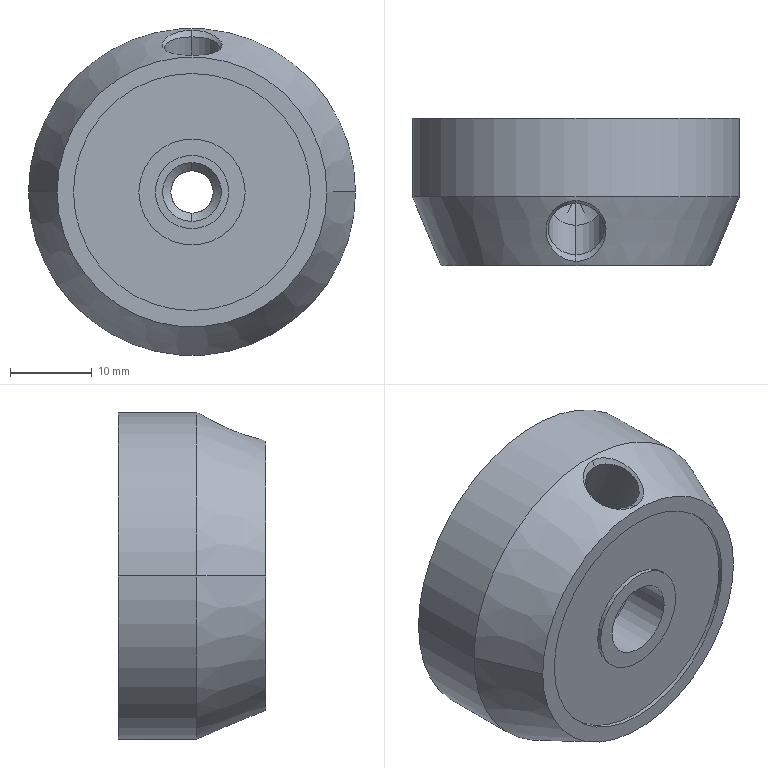Part | SolidWorks | features ICE 8, Chamfer 1, ExtruRefSurface 1, HoleWzd 1, Revolution 1 | 1 solid | 48 faces | box 40 x 18 x 40 mm | volume 16236 mm3 | cylinder 27 | plane 13 | cone 8 | commonest cylinder face diameters 6 x4 5 x3 5.2 x2 6.8 x2 7 x2 8 x2
STEP:
#1=CARTESIAN_POINT('',(20.,2.785,10.327));
#2=VERTEX_POINT('',#1);
#3=CARTESIAN_POINT('',(20.,-3.492,7.712));
#4=VERTEX_POINT('',#3);
#5=CARTESIAN_POINT('',(20.,-0.3538,9.019));
#6=DIRECTION('',(0.,-0.3846,0.9231));
#7=DIRECTION('',(0.,-0.9231,-0.3846));
#8=AXIS2_PLACEMENT_3D('',#5,#6,#7);
#9=CIRCLE('',#8,3.4);
#10=EDGE_CURVE('',#2,#4,#9,.T.);
#11=ORIENTED_EDGE('',*,*,#10,.F.);
#12=CARTESIAN_POINT('',(20.,-0.8212,18.981));
#13=VERTEX_POINT('',#12);
#14=CARTESIAN_POINT('',(20.,-1.062,19.558));
#15=DIRECTION('',(0.,-0.3846,0.9231));
#16=VECTOR('',#15,1000.);
#17=LINE('',#14,#16);
#18=EDGE_CURVE('',#2,#13,#17,.T.);
#19=ORIENTED_EDGE('',*,*,#18,.T.);
#20=CARTESIAN_POINT('',(20.,-7.098,16.365));
#21=VERTEX_POINT('',#20);
#22=CARTESIAN_POINT('',(20.,-3.96,17.673));
#23=DIRECTION('',(0.,-0.3846,0.9231));
#24=DIRECTION('',(0.,-0.9231,-0.3846));
#25=AXIS2_PLACEMENT_3D('',#22,#23,#24);
#26=CIRCLE('',#25,3.4);
#27=EDGE_CURVE('',#13,#21,#26,.T.);
#28=ORIENTED_EDGE('',*,*,#27,.T.);
#29=CARTESIAN_POINT('',(20.,-7.338,16.942));
#30=DIRECTION('',(0.,-0.3846,0.9231));
#31=VECTOR('',#30,1000.);
#32=LINE('',#29,#31);
#33=EDGE_CURVE('',#4,#21,#32,.T.);
#34=ORIENTED_EDGE('',*,*,#33,.F.);
#35=EDGE_LOOP('',(#11,#19,#28,#34));
#36=FACE_OUTER_BOUND('',#35,.T.);
#37=CARTESIAN_POINT('',(20.,-4.2,18.25));
#38=DIRECTION('',(0.,-0.3846,0.9231));
#39=DIRECTION('',(0.,-0.9231,-0.3846));
#40=AXIS2_PLACEMENT_3D('',#37,#38,#39);
#41=CYLINDRICAL_SURFACE('',#40,3.4);
#42=ADVANCED_FACE('',(#36),#41,.F.);
#43=CARTESIAN_POINT('',(20.,0.4319,7.133));
#44=VERTEX_POINT('',#43);
#45=CARTESIAN_POINT('',(20.,-3.492,7.712));
#46=DIRECTION('',(0.,-0.9893,0.1457));
#47=VECTOR('',#46,1000.);
#48=LINE('',#45,#47);
#49=EDGE_CURVE('',#44,#4,#48,.T.);
#50=ORIENTED_EDGE('',*,*,#49,.F.);
#51=CARTESIAN_POINT('',(20.,2.785,10.327));
#52=DIRECTION('',(0.,0.5931,0.8051));
#53=VECTOR('',#52,1000.);
#54=LINE('',#51,#53);
#55=EDGE_CURVE('',#44,#2,#54,.T.);
#56=ORIENTED_EDGE('',*,*,#55,.T.);
#57=ORIENTED_EDGE('',*,*,#10,.T.);
#58=EDGE_LOOP('',(#50,#56,#57));
#59=FACE_OUTER_BOUND('',#58,.T.);
#60=CARTESIAN_POINT('',(20.,-0.3538,9.019));
#61=DIRECTION('',(0.,-0.3846,0.9231));
#62=DIRECTION('',(0.,-0.9231,-0.3846));
#63=AXIS2_PLACEMENT_3D('',#60,#61,#62);
#64=CONICAL_SURFACE('',#63,3.4,1.03);
#65=ADVANCED_FACE('',(#59),#64,.F.);
#66=ORIENTED_EDGE('',*,*,#27,.F.);
#67=CARTESIAN_POINT('',(20.,-0.4846,19.798));
#68=VERTEX_POINT('',#67);
#69=CARTESIAN_POINT('',(20.,-0.4846,19.798));
#70=DIRECTION('',(0.,0.3807,0.9247));
#71=VECTOR('',#70,1000.);
#72=LINE('',#69,#71);
#73=EDGE_CURVE('',#13,#68,#72,.T.);
#74=ORIENTED_EDGE('',*,*,#73,.T.);
#75=CARTESIAN_POINT('',(20.,-7.915,16.702));
#76=VERTEX_POINT('',#75);
#77=CARTESIAN_POINT('',(20.,-7.915,16.702));
#78=CARTESIAN_POINT('',(19.748,-7.915,16.702));
#79=CARTESIAN_POINT('',(19.492,-7.886,16.708));
#80=CARTESIAN_POINT('',(19.001,-7.772,16.734));
#81=CARTESIAN_POINT('',(18.762,-7.688,16.753));
#82=CARTESIAN_POINT('',(18.304,-7.469,16.804));
#83=CARTESIAN_POINT('',(18.091,-7.338,16.836));
#84=CARTESIAN_POINT('',(17.693,-7.035,16.913));
#85=CARTESIAN_POINT('',(17.508,-6.863,16.959));
#86=CARTESIAN_POINT('',(17.176,-6.492,17.064));
#87=CARTESIAN_POINT('',(17.029,-6.292,17.123));
#88=CARTESIAN_POINT('',(16.776,-5.877,17.253));
#89=CARTESIAN_POINT('',(16.67,-5.66,17.324));
#90=CARTESIAN_POINT('',(16.497,-5.211,17.481));
#91=CARTESIAN_POINT('',(16.431,-4.98,17.566));
#92=CARTESIAN_POINT('',(16.343,-4.518,17.745));
#93=CARTESIAN_POINT('',(16.321,-4.286,17.839));
#94=CARTESIAN_POINT('',(16.319,-3.818,18.037));
#95=CARTESIAN_POINT('',(16.341,-3.587,18.14));
#96=CARTESIAN_POINT('',(16.427,-3.139,18.348));
#97=CARTESIAN_POINT('',(16.491,-2.919,18.453));
#98=CARTESIAN_POINT('',(16.665,-2.491,18.667));
#99=CARTESIAN_POINT('',(16.772,-2.288,18.772));
#100=CARTESIAN_POINT('',(17.025,-1.906,18.975));
#101=CARTESIAN_POINT('',(17.173,-1.725,19.074));
#102=CARTESIAN_POINT('',(17.508,-1.391,19.26));
#103=CARTESIAN_POINT('',(17.691,-1.242,19.346));
#104=CARTESIAN_POINT('',(18.089,-0.9786,19.5));
#105=CARTESIAN_POINT('',(18.307,-0.863,19.569));
#106=CARTESIAN_POINT('',(18.764,-0.6766,19.681));
#107=CARTESIAN_POINT('',(19.001,-0.6058,19.724));
#108=CARTESIAN_POINT('',(19.492,-0.5095,19.783));
#109=CARTESIAN_POINT('',(19.748,-0.4846,19.798));
#110=CARTESIAN_POINT('',(20.,-0.4846,19.798));
#111=B_SPLINE_CURVE_WITH_KNOTS('',3,(#77,#78,#79,#80,#81,#82,#83,#84,#85,#86,#87,#88,#89,#90,#91,#92,#93,#94,#95,#96,#97,#98,#99,#100,#101,#102,#103,#104,#105,#106,#107,#108,#109,#110),.UNSPECIFIED.,.F.,.F.,(4,2,2,2,2,2,2,2,2,2,2,2,2,2,2,2,4),(0.02082,0.02157,0.02232,0.02308,0.02383,0.02458,0.02534,0.02609,0.02684,0.0276,0.02835,0.0291,0.02986,0.03061,0.03136,0.03212,0.03287),.UNSPECIFIED.);
#112=EDGE_CURVE('',#76,#68,#111,.T.);
#113=ORIENTED_EDGE('',*,*,#112,.F.);
#114=CARTESIAN_POINT('',(20.,-7.915,16.702));
#115=DIRECTION('',(0.,-0.9247,0.3807));
#116=VECTOR('',#115,1000.);
#117=LINE('',#114,#116);
#118=EDGE_CURVE('',#21,#76,#117,.T.);
#119=ORIENTED_EDGE('',*,*,#118,.F.);
#120=EDGE_LOOP('',(#66,#74,#113,#119));
#121=FACE_OUTER_BOUND('',#120,.T.);
#122=CARTESIAN_POINT('',(20.,-4.2,18.25));
#123=DIRECTION('',(0.,-0.3846,0.9231));
#124=DIRECTION('',(0.,-0.9231,-0.3846));
#125=AXIS2_PLACEMENT_3D('',#122,#123,#124);
#126=CONICAL_SURFACE('',#125,4.025,0.7854);
#127=ADVANCED_FACE('',(#121),#126,.F.);
#128=CARTESIAN_POINT('',(26.5,-7.9,0.));
#129=VERTEX_POINT('',#128);
#130=CARTESIAN_POINT('',(13.5,-7.9,0.));
#131=VERTEX_POINT('',#130);
#132=CARTESIAN_POINT('',(20.,-7.9,0.));
#133=DIRECTION('',(0.,-1.,0.));
#134=DIRECTION('',(1.,0.,0.));
#135=AXIS2_PLACEMENT_3D('',#132,#133,#134);
#136=CIRCLE('',#135,6.5);
#137=EDGE_CURVE('',#129,#131,#136,.T.);
#138=ORIENTED_EDGE('',*,*,#137,.T.);
#139=CARTESIAN_POINT('',(13.5,-8.4,0.));
#140=VERTEX_POINT('',#139);
#141=CARTESIAN_POINT('',(13.5,-7.9,0.));
#142=DIRECTION('',(0.,-1.,0.));
#143=VECTOR('',#142,1000.);
#144=LINE('',#141,#143);
#145=EDGE_CURVE('',#131,#140,#144,.T.);
#146=ORIENTED_EDGE('',*,*,#145,.T.);
#147=CARTESIAN_POINT('',(26.5,-8.4,0.));
#148=VERTEX_POINT('',#147);
#149=CARTESIAN_POINT('',(20.,-8.4,0.));
#150=DIRECTION('',(0.,-1.,0.));
#151=DIRECTION('',(1.,0.,0.));
#152=AXIS2_PLACEMENT_3D('',#149,#150,#151);
#153=CIRCLE('',#152,6.5);
#154=EDGE_CURVE('',#148,#140,#153,.T.);
#155=ORIENTED_EDGE('',*,*,#154,.F.);
#156=CARTESIAN_POINT('',(26.5,-7.9,0.));
#157=DIRECTION('',(0.,-1.,0.));
#158=VECTOR('',#157,1000.);
#159=LINE('',#156,#158);
#160=EDGE_CURVE('',#129,#148,#159,.T.);
#161=ORIENTED_EDGE('',*,*,#160,.F.);
#162=EDGE_LOOP('',(#138,#146,#155,#161));
#163=FACE_OUTER_BOUND('',#162,.T.);
#164=CARTESIAN_POINT('',(20.,-7.9,0.));
#165=DIRECTION('',(0.,-1.,0.));
#166=DIRECTION('',(1.,0.,0.));
#167=AXIS2_PLACEMENT_3D('',#164,#165,#166);
#168=CYLINDRICAL_SURFACE('',#167,6.5);
#169=ADVANCED_FACE('',(#163),#168,.T.);
#170=CARTESIAN_POINT('',(5.5,-7.9,0.));
#171=VERTEX_POINT('',#170);
#172=CARTESIAN_POINT('',(34.5,-7.9,0.));
#173=VERTEX_POINT('',#172);
#174=CARTESIAN_POINT('',(20.,-7.9,0.));
#175=DIRECTION('',(0.,-1.,0.));
#176=DIRECTION('',(1.,0.,0.));
#177=AXIS2_PLACEMENT_3D('',#174,#175,#176);
#178=CIRCLE('',#177,14.5);
#179=EDGE_CURVE('',#171,#173,#178,.T.);
#180=ORIENTED_EDGE('',*,*,#179,.F.);
#181=CARTESIAN_POINT('',(5.5,-8.4,0.));
#182=VERTEX_POINT('',#181);
#183=CARTESIAN_POINT('',(5.5,-7.9,0.));
#184=DIRECTION('',(0.,-1.,0.));
#185=VECTOR('',#184,1000.);
#186=LINE('',#183,#185);
#187=EDGE_CURVE('',#171,#182,#186,.T.);
#188=ORIENTED_EDGE('',*,*,#187,.T.);
#189=CARTESIAN_POINT('',(34.5,-8.4,0.));
#190=VERTEX_POINT('',#189);
#191=CARTESIAN_POINT('',(20.,-8.4,0.));
#192=DIRECTION('',(0.,-1.,0.));
#193=DIRECTION('',(1.,0.,0.));
#194=AXIS2_PLACEMENT_3D('',#191,#192,#193);
#195=CIRCLE('',#194,14.5);
#196=EDGE_CURVE('',#182,#190,#195,.T.);
#197=ORIENTED_EDGE('',*,*,#196,.T.);
#198=CARTESIAN_POINT('',(34.5,-7.9,0.));
#199=DIRECTION('',(0.,-1.,0.));
#200=VECTOR('',#199,1000.);
#201=LINE('',#198,#200);
#202=EDGE_CURVE('',#173,#190,#201,.T.);
#203=ORIENTED_EDGE('',*,*,#202,.F.);
#204=EDGE_LOOP('',(#180,#188,#197,#203));
#205=FACE_OUTER_BOUND('',#204,.T.);
#206=CARTESIAN_POINT('',(20.,-7.9,0.));
#207=DIRECTION('',(0.,-1.,0.));
#208=DIRECTION('',(1.,0.,0.));
#209=AXIS2_PLACEMENT_3D('',#206,#207,#208);
#210=CYLINDRICAL_SURFACE('',#209,14.5);
#211=ADVANCED_FACE('',(#205),#210,.F.);
#212=CARTESIAN_POINT('',(20.,-1.4,2.6));
#213=VERTEX_POINT('',#212);
#214=CARTESIAN_POINT('',(17.4,-1.4,0.));
#215=VERTEX_POINT('',#214);
#216=CARTESIAN_POINT('',(20.,-1.4,0.));
#217=DIRECTION('',(0.,-1.,0.));
#218=DIRECTION('',(0.,0.,-1.));
#219=AXIS2_PLACEMENT_3D('',#216,#217,#218);
#220=CIRCLE('',#219,2.6);
#221=EDGE_CURVE('',#213,#215,#220,.T.);
#222=ORIENTED_EDGE('',*,*,#221,.F.);
#223=CARTESIAN_POINT('',(20.,-2.4,3.6));
#224=VERTEX_POINT('',#223);
#225=CARTESIAN_POINT('',(20.,-1.4,2.6));
#226=DIRECTION('',(0.,-0.7071,0.7071));
#227=VECTOR('',#226,1000.);
#228=LINE('',#225,#227);
#229=EDGE_CURVE('',#213,#224,#228,.T.);
#230=ORIENTED_EDGE('',*,*,#229,.T.);
#231=CARTESIAN_POINT('',(20.,-2.4,-3.6));
#232=VERTEX_POINT('',#231);
#233=CARTESIAN_POINT('',(20.,-2.4,0.));
#234=DIRECTION('',(0.,1.,0.));
#235=DIRECTION('',(1.,0.,0.));
#236=AXIS2_PLACEMENT_3D('',#233,#234,#235);
#237=CIRCLE('',#236,3.6);
#238=EDGE_CURVE('',#232,#224,#237,.T.);
#239=ORIENTED_EDGE('',*,*,#238,.F.);
#240=CARTESIAN_POINT('',(20.,-1.4,-2.6));
#241=VERTEX_POINT('',#240);
#242=CARTESIAN_POINT('',(20.,-1.4,-2.6));
#243=DIRECTION('',(0.,-0.7071,-0.7071));
#244=VECTOR('',#243,1000.);
#245=LINE('',#242,#244);
#246=EDGE_CURVE('',#241,#232,#245,.T.);
#247=ORIENTED_EDGE('',*,*,#246,.F.);
#248=CARTESIAN_POINT('',(20.,-1.4,0.));
#249=DIRECTION('',(0.,-1.,0.));
#250=DIRECTION('',(0.,0.,-1.));
#251=AXIS2_PLACEMENT_3D('',#248,#249,#250);
#252=CIRCLE('',#251,2.6);
#253=EDGE_CURVE('',#215,#241,#252,.T.);
#254=ORIENTED_EDGE('',*,*,#253,.F.);
#255=EDGE_LOOP('',(#222,#230,#239,#247,#254));
#256=FACE_OUTER_BOUND('',#255,.T.);
#257=CARTESIAN_POINT('',(20.,-1.4,0.));
#258=DIRECTION('',(0.,-1.,0.));
#259=DIRECTION('',(0.,0.,-1.));
#260=AXIS2_PLACEMENT_3D('',#257,#258,#259);
#261=CONICAL_SURFACE('',#260,2.6,0.7854);
#262=ADVANCED_FACE('',(#256),#261,.F.);
#263=ORIENTED_EDGE('',*,*,#253,.T.);
#264=CARTESIAN_POINT('',(22.6,-1.4,0.));
#265=VERTEX_POINT('',#264);
#266=CARTESIAN_POINT('',(20.,-1.4,0.));
#267=DIRECTION('',(0.,-1.,0.));
#268=DIRECTION('',(0.,0.,-1.));
#269=AXIS2_PLACEMENT_3D('',#266,#267,#268);
#270=CIRCLE('',#269,2.6);
#271=EDGE_CURVE('',#241,#265,#270,.T.);
#272=ORIENTED_EDGE('',*,*,#271,.T.);
#273=CARTESIAN_POINT('',(22.6,0.6,0.));
#274=VERTEX_POINT('',#273);
#275=CARTESIAN_POINT('',(22.6,-8.4,0.));
#276=DIRECTION('',(0.,1.,0.));
#277=VECTOR('',#276,1000.);
#278=LINE('',#275,#277);
#279=EDGE_CURVE('',#265,#274,#278,.T.);
#280=ORIENTED_EDGE('',*,*,#279,.T.);
#281=CARTESIAN_POINT('',(17.4,0.6,0.));
#282=VERTEX_POINT('',#281);
#283=CARTESIAN_POINT('',(20.,0.6,0.));
#284=DIRECTION('',(0.,1.,0.));
#285=DIRECTION('',(-1.,0.,0.));
#286=AXIS2_PLACEMENT_3D('',#283,#284,#285);
#287=CIRCLE('',#286,2.6);
#288=EDGE_CURVE('',#274,#282,#287,.T.);
#289=ORIENTED_EDGE('',*,*,#288,.T.);
#290=CARTESIAN_POINT('',(17.4,-8.4,0.));
#291=DIRECTION('',(0.,1.,0.));
#292=VECTOR('',#291,1000.);
#293=LINE('',#290,#292);
#294=EDGE_CURVE('',#215,#282,#293,.T.);
#295=ORIENTED_EDGE('',*,*,#294,.F.);
#296=EDGE_LOOP('',(#263,#272,#280,#289,#295));
#297=FACE_OUTER_BOUND('',#296,.T.);
#298=CARTESIAN_POINT('',(20.,-8.4,0.));
#299=DIRECTION('',(0.,1.,0.));
#300=DIRECTION('',(-1.,0.,0.));
#301=AXIS2_PLACEMENT_3D('',#298,#299,#300);
#302=CYLINDRICAL_SURFACE('',#301,2.6);
#303=ADVANCED_FACE('',(#297),#302,.F.);
#304=CARTESIAN_POINT('',(23.5,0.6,0.));
#305=VERTEX_POINT('',#304);
#306=CARTESIAN_POINT('',(16.5,0.6,0.));
#307=VERTEX_POINT('',#306);
#308=CARTESIAN_POINT('',(20.,0.6,0.));
#309=DIRECTION('',(0.,1.,0.));
#310=DIRECTION('',(-1.,0.,0.));
#311=AXIS2_PLACEMENT_3D('',#308,#309,#310);
#312=CIRCLE('',#311,3.5);
#313=EDGE_CURVE('',#305,#307,#312,.T.);
#314=ORIENTED_EDGE('',*,*,#313,.F.);
#315=CARTESIAN_POINT('',(23.5,3.1,0.));
#316=VERTEX_POINT('',#315);
#317=CARTESIAN_POINT('',(23.5,0.6,0.));
#318=DIRECTION('',(0.,1.,0.));
#319=VECTOR('',#318,1000.);
#320=LINE('',#317,#319);
#321=EDGE_CURVE('',#305,#316,#320,.T.);
#322=ORIENTED_EDGE('',*,*,#321,.T.);
#323=CARTESIAN_POINT('',(16.5,3.1,0.));
#324=VERTEX_POINT('',#323);
#325=CARTESIAN_POINT('',(20.,3.1,0.));
#326=DIRECTION('',(0.,1.,0.));
#327=DIRECTION('',(-1.,0.,0.));
#328=AXIS2_PLACEMENT_3D('',#325,#326,#327);
#329=CIRCLE('',#328,3.5);
#330=EDGE_CURVE('',#316,#324,#329,.T.);
#331=ORIENTED_EDGE('',*,*,#330,.T.);
#332=CARTESIAN_POINT('',(16.5,0.6,0.));
#333=DIRECTION('',(0.,1.,0.));
#334=VECTOR('',#333,1000.);
#335=LINE('',#332,#334);
#336=EDGE_CURVE('',#307,#324,#335,.T.);
#337=ORIENTED_EDGE('',*,*,#336,.F.);
#338=EDGE_LOOP('',(#314,#322,#331,#337));
#339=FACE_OUTER_BOUND('',#338,.T.);
#340=CARTESIAN_POINT('',(20.,0.6,0.));
#341=DIRECTION('',(0.,1.,0.));
#342=DIRECTION('',(-1.,0.,0.));
#343=AXIS2_PLACEMENT_3D('',#340,#341,#342);
#344=CYLINDRICAL_SURFACE('',#343,3.5);
#345=ADVANCED_FACE('',(#339),#344,.F.);
#346=CARTESIAN_POINT('',(15.5,-2.4,0.));
#347=VERTEX_POINT('',#346);
#348=CARTESIAN_POINT('',(24.5,-2.4,0.));
#349=VERTEX_POINT('',#348);
#350=CARTESIAN_POINT('',(20.,-2.4,0.));
#351=DIRECTION('',(0.,-1.,0.));
#352=DIRECTION('',(1.,0.,0.));
#353=AXIS2_PLACEMENT_3D('',#350,#351,#352);
#354=CIRCLE('',#353,4.5);
#355=EDGE_CURVE('',#347,#349,#354,.T.);
#356=ORIENTED_EDGE('',*,*,#355,.F.);
#357=CARTESIAN_POINT('',(15.5,-8.4,0.));
#358=VERTEX_POINT('',#357);
#359=CARTESIAN_POINT('',(15.5,-2.4,0.));
#360=DIRECTION('',(0.,-1.,0.));
#361=VECTOR('',#360,1000.);
#362=LINE('',#359,#361);
#363=EDGE_CURVE('',#347,#358,#362,.T.);
#364=ORIENTED_EDGE('',*,*,#363,.T.);
#365=CARTESIAN_POINT('',(24.5,-8.4,0.));
#366=VERTEX_POINT('',#365);
#367=CARTESIAN_POINT('',(20.,-8.4,0.));
#368=DIRECTION('',(0.,-1.,0.));
#369=DIRECTION('',(1.,0.,0.));
#370=AXIS2_PLACEMENT_3D('',#367,#368,#369);
#371=CIRCLE('',#370,4.5);
#372=EDGE_CURVE('',#358,#366,#371,.T.);
#373=ORIENTED_EDGE('',*,*,#372,.T.);
#374=CARTESIAN_POINT('',(24.5,-2.4,0.));
#375=DIRECTION('',(0.,-1.,0.));
#376=VECTOR('',#375,1000.);
#377=LINE('',#374,#376);
#378=EDGE_CURVE('',#349,#366,#377,.T.);
#379=ORIENTED_EDGE('',*,*,#378,.F.);
#380=EDGE_LOOP('',(#356,#364,#373,#379));
#381=FACE_OUTER_BOUND('',#380,.T.);
#382=CARTESIAN_POINT('',(20.,-2.4,0.));
#383=DIRECTION('',(0.,-1.,0.));
#384=DIRECTION('',(1.,0.,0.));
#385=AXIS2_PLACEMENT_3D('',#382,#383,#384);
#386=CYLINDRICAL_SURFACE('',#385,4.5);
#387=ADVANCED_FACE('',(#381),#386,.F.);
#388=CARTESIAN_POINT('',(9.,-3.4,0.));
#389=VERTEX_POINT('',#388);
#390=CARTESIAN_POINT('',(3.,-3.4,0.));
#391=VERTEX_POINT('',#390);
#392=CARTESIAN_POINT('',(6.,-3.4,0.));
#393=DIRECTION('',(0.,1.,0.));
#394=DIRECTION('',(-1.,0.,0.));
#395=AXIS2_PLACEMENT_3D('',#392,#393,#394);
#396=CIRCLE('',#395,3.);
#397=EDGE_CURVE('',#389,#391,#396,.T.);
#398=ORIENTED_EDGE('',*,*,#397,.F.);
#399=CARTESIAN_POINT('',(9.,7.6,0.));
#400=VERTEX_POINT('',#399);
#401=CARTESIAN_POINT('',(9.,-3.4,0.));
#402=DIRECTION('',(0.,1.,0.));
#403=VECTOR('',#402,1000.);
#404=LINE('',#401,#403);
#405=EDGE_CURVE('',#389,#400,#404,.T.);
#406=ORIENTED_EDGE('',*,*,#405,.T.);
#407=CARTESIAN_POINT('',(3.,7.6,0.));
#408=VERTEX_POINT('',#407);
#409=CARTESIAN_POINT('',(6.,7.6,0.));
#410=DIRECTION('',(0.,1.,0.));
#411=DIRECTION('',(-1.,0.,0.));
#412=AXIS2_PLACEMENT_3D('',#409,#410,#411);
#413=CIRCLE('',#412,3.);
#414=EDGE_CURVE('',#400,#408,#413,.T.);
#415=ORIENTED_EDGE('',*,*,#414,.T.);
#416=CARTESIAN_POINT('',(3.,-3.4,0.));
#417=DIRECTION('',(0.,1.,0.));
#418=VECTOR('',#417,1000.);
#419=LINE('',#416,#418);
#420=EDGE_CURVE('',#391,#408,#419,.T.);
#421=ORIENTED_EDGE('',*,*,#420,.F.);
#422=EDGE_LOOP('',(#398,#406,#415,#421));
#423=FACE_OUTER_BOUND('',#422,.T.);
#424=CARTESIAN_POINT('',(6.,-3.4,0.));
#425=DIRECTION('',(0.,1.,0.));
#426=DIRECTION('',(-1.,0.,0.));
#427=AXIS2_PLACEMENT_3D('',#424,#425,#426);
#428=CYLINDRICAL_SURFACE('',#427,3.);
#429=ADVANCED_FACE('',(#423),#428,.F.);
#430=CARTESIAN_POINT('',(37.,-3.4,0.));
#431=VERTEX_POINT('',#430);
#432=CARTESIAN_POINT('',(31.,-3.4,0.));
#433=VERTEX_POINT('',#432);
#434=CARTESIAN_POINT('',(34.,-3.4,0.));
#435=DIRECTION('',(0.,1.,0.));
#436=DIRECTION('',(1.,0.,0.));
#437=AXIS2_PLACEMENT_3D('',#434,#435,#436);
#438=CIRCLE('',#437,3.);
#439=EDGE_CURVE('',#431,#433,#438,.T.);
#440=ORIENTED_EDGE('',*,*,#439,.F.);
#441=CARTESIAN_POINT('',(37.,7.6,0.));
#442=VERTEX_POINT('',#441);
#443=CARTESIAN_POINT('',(37.,-3.4,0.));
#444=DIRECTION('',(0.,1.,0.));
#445=VECTOR('',#444,1000.);
#446=LINE('',#443,#445);
#447=EDGE_CURVE('',#431,#442,#446,.T.);
#448=ORIENTED_EDGE('',*,*,#447,.T.);
#449=CARTESIAN_POINT('',(31.,7.6,0.));
#450=VERTEX_POINT('',#449);
#451=CARTESIAN_POINT('',(34.,7.6,0.));
#452=DIRECTION('',(0.,1.,0.));
#453=DIRECTION('',(1.,0.,0.));
#454=AXIS2_PLACEMENT_3D('',#451,#452,#453);
#455=CIRCLE('',#454,3.);
#456=EDGE_CURVE('',#442,#450,#455,.T.);
#457=ORIENTED_EDGE('',*,*,#456,.T.);
#458=CARTESIAN_POINT('',(31.,-3.4,0.));
#459=DIRECTION('',(0.,1.,0.));
#460=VECTOR('',#459,1000.);
#461=LINE('',#458,#460);
#462=EDGE_CURVE('',#433,#450,#461,.T.);
#463=ORIENTED_EDGE('',*,*,#462,.F.);
#464=EDGE_LOOP('',(#440,#448,#457,#463));
#465=FACE_OUTER_BOUND('',#464,.T.);
#466=CARTESIAN_POINT('',(34.,-3.4,0.));
#467=DIRECTION('',(0.,1.,0.));
#468=DIRECTION('',(-1.,0.,0.));
#469=AXIS2_PLACEMENT_3D('',#466,#467,#468);
#470=CYLINDRICAL_SURFACE('',#469,3.);
#471=ADVANCED_FACE('',(#465),#470,.F.);
#472=CARTESIAN_POINT('',(7.601,4.1,-9.899));
#473=VERTEX_POINT('',#472);
#474=CARTESIAN_POINT('',(11.868,4.1,-8.132));
#475=VERTEX_POINT('',#474);
#476=CARTESIAN_POINT('',(10.101,4.1,-9.899));
#477=DIRECTION('',(0.,1.,0.));
#478=DIRECTION('',(-1.,0.,0.));
#479=AXIS2_PLACEMENT_3D('',#476,#477,#478);
#480=CIRCLE('',#479,2.5);
#481=EDGE_CURVE('',#473,#475,#480,.T.);
#482=ORIENTED_EDGE('',*,*,#481,.F.);
#483=CARTESIAN_POINT('',(7.601,7.6,-9.899));
#484=VERTEX_POINT('',#483);
#485=CARTESIAN_POINT('',(7.601,4.1,-9.899));
#486=DIRECTION('',(0.,1.,0.));
#487=VECTOR('',#486,1000.);
#488=LINE('',#485,#487);
#489=EDGE_CURVE('',#473,#484,#488,.T.);
#490=ORIENTED_EDGE('',*,*,#489,.T.);
#491=CARTESIAN_POINT('',(11.868,7.6,-8.132));
#492=VERTEX_POINT('',#491);
#493=CARTESIAN_POINT('',(10.101,7.6,-9.899));
#494=DIRECTION('',(0.,1.,0.));
#495=DIRECTION('',(-1.,0.,0.));
#496=AXIS2_PLACEMENT_3D('',#493,#494,#495);
#497=CIRCLE('',#496,2.5);
#498=EDGE_CURVE('',#484,#492,#497,.T.);
#499=ORIENTED_EDGE('',*,*,#498,.T.);
#500=CARTESIAN_POINT('',(11.868,4.1,-8.132));
#501=DIRECTION('',(0.,1.,0.));
#502=VECTOR('',#501,1000.);
#503=LINE('',#500,#502);
#504=EDGE_CURVE('',#475,#492,#503,.T.);
#505=ORIENTED_EDGE('',*,*,#504,.F.);
#506=EDGE_LOOP('',(#482,#490,#499,#505));
#507=FACE_OUTER_BOUND('',#506,.T.);
#508=CARTESIAN_POINT('',(10.101,4.1,-9.899));
#509=DIRECTION('',(0.,1.,0.));
#510=DIRECTION('',(-1.,0.,0.));
#511=AXIS2_PLACEMENT_3D('',#508,#509,#510);
#512=CYLINDRICAL_SURFACE('',#511,2.5);
#513=ADVANCED_FACE('',(#507),#512,.F.);
#514=CARTESIAN_POINT('',(20.,7.6,0.));
#515=DIRECTION('',(0.,1.,0.));
#516=DIRECTION('',(-1.,0.,0.));
#517=AXIS2_PLACEMENT_3D('',#514,#515,#516);
#518=CIRCLE('',#517,17.);
#519=EDGE_CURVE('',#442,#408,#518,.T.);
#520=ORIENTED_EDGE('',*,*,#519,.F.);
#521=CARTESIAN_POINT('',(37.,9.6,0.));
#522=VERTEX_POINT('',#521);
#523=CARTESIAN_POINT('',(37.,7.6,0.));
#524=DIRECTION('',(0.,1.,0.));
#525=VECTOR('',#524,1000.);
#526=LINE('',#523,#525);
#527=EDGE_CURVE('',#442,#522,#526,.T.);
#528=ORIENTED_EDGE('',*,*,#527,.T.);
#529=CARTESIAN_POINT('',(3.,9.6,0.));
#530=VERTEX_POINT('',#529);
#531=CARTESIAN_POINT('',(20.,9.6,0.));
#532=DIRECTION('',(0.,1.,0.));
#533=DIRECTION('',(-1.,0.,0.));
#534=AXIS2_PLACEMENT_3D('',#531,#532,#533);
#535=CIRCLE('',#534,17.);
#536=EDGE_CURVE('',#522,#530,#535,.T.);
#537=ORIENTED_EDGE('',*,*,#536,.T.);
#538=CARTESIAN_POINT('',(3.,7.6,0.));
#539=DIRECTION('',(0.,1.,0.));
#540=VECTOR('',#539,1000.);
#541=LINE('',#538,#540);
#542=EDGE_CURVE('',#408,#530,#541,.T.);
#543=ORIENTED_EDGE('',*,*,#542,.F.);
#544=EDGE_LOOP('',(#520,#528,#537,#543));
#545=FACE_OUTER_BOUND('',#544,.T.);
#546=CARTESIAN_POINT('',(20.,7.6,0.));
#547=DIRECTION('',(0.,1.,0.));
#548=DIRECTION('',(-1.,0.,0.));
#549=AXIS2_PLACEMENT_3D('',#546,#547,#548);
#550=CYLINDRICAL_SURFACE('',#549,17.);
#551=ADVANCED_FACE('',(#545),#550,.F.);
#552=ORIENTED_EDGE('',*,*,#112,.T.);
#553=CARTESIAN_POINT('',(20.,-0.4846,19.798));
#554=CARTESIAN_POINT('',(20.252,-0.4846,19.798));
#555=CARTESIAN_POINT('',(20.503,-0.5087,19.783));
#556=CARTESIAN_POINT('',(21.,-0.606,19.724));
#557=CARTESIAN_POINT('',(21.238,-0.6774,19.68));
#558=CARTESIAN_POINT('',(21.694,-0.8637,19.568));
#559=CARTESIAN_POINT('',(21.913,-0.9798,19.499));
#560=CARTESIAN_POINT('',(22.313,-1.245,19.344));
#561=CARTESIAN_POINT('',(22.497,-1.396,19.258));
#562=CARTESIAN_POINT('',(22.832,-1.731,19.07));
#563=CARTESIAN_POINT('',(22.979,-1.911,18.972));
#564=CARTESIAN_POINT('',(23.233,-2.296,18.767));
#565=CARTESIAN_POINT('',(23.341,-2.503,18.661));
#566=CARTESIAN_POINT('',(23.512,-2.929,18.449));
#567=CARTESIAN_POINT('',(23.576,-3.148,18.343));
#568=CARTESIAN_POINT('',(23.661,-3.6,18.134));
#569=CARTESIAN_POINT('',(23.682,-3.834,18.031));
#570=CARTESIAN_POINT('',(23.679,-4.298,17.834));
#571=CARTESIAN_POINT('',(23.656,-4.53,17.74));
#572=CARTESIAN_POINT('',(23.566,-4.994,17.561));
#573=CARTESIAN_POINT('',(23.499,-5.226,17.476));
#574=CARTESIAN_POINT('',(23.325,-5.672,17.32));
#575=CARTESIAN_POINT('',(23.218,-5.888,17.249));
#576=CARTESIAN_POINT('',(22.962,-6.306,17.119));
#577=CARTESIAN_POINT('',(22.813,-6.505,17.06));
#578=CARTESIAN_POINT('',(22.485,-6.871,16.957));
#579=CARTESIAN_POINT('',(22.303,-7.039,16.912));
#580=CARTESIAN_POINT('',(21.903,-7.342,16.835));
#581=CARTESIAN_POINT('',(21.687,-7.474,16.803));
#582=CARTESIAN_POINT('',(21.237,-7.688,16.753));
#583=CARTESIAN_POINT('',(20.998,-7.773,16.733));
#584=CARTESIAN_POINT('',(20.502,-7.887,16.708));
#585=CARTESIAN_POINT('',(20.252,-7.915,16.702));
#586=CARTESIAN_POINT('',(20.,-7.915,16.702));
#587=B_SPLINE_CURVE_WITH_KNOTS('',3,(#553,#554,#555,#556,#557,#558,#559,#560,#561,#562,#563,#564,#565,#566,#567,#568,#569,#570,#571,#572,#573,#574,#575,#576,#577,#578,#579,#580,#581,#582,#583,#584,#585,#586),.UNSPECIFIED.,.F.,.F.,(4,2,2,2,2,2,2,2,2,2,2,2,2,2,2,2,4),(0.008758,0.009511,0.01027,0.01102,0.01177,0.01253,0.01328,0.01403,0.01479,0.01554,0.01629,0.01705,0.0178,0.01856,0.01931,0.02006,0.02082),.UNSPECIFIED.);
#588=EDGE_CURVE('',#68,#76,#587,.T.);
#589=ORIENTED_EDGE('',*,*,#588,.T.);
#590=EDGE_LOOP('',(#552,#589));
#591=FACE_BOUND('',#590,.T.);
#592=CARTESIAN_POINT('',(36.5,-8.4,0.));
#593=VERTEX_POINT('',#592);
#594=CARTESIAN_POINT('',(3.5,-8.4,0.));
#595=VERTEX_POINT('',#594);
#596=CARTESIAN_POINT('',(20.,-8.4,0.));
#597=DIRECTION('',(0.,-1.,0.));
#598=DIRECTION('',(1.,0.,0.));
#599=AXIS2_PLACEMENT_3D('',#596,#597,#598);
#600=CIRCLE('',#599,16.5);
#601=EDGE_CURVE('',#593,#595,#600,.T.);
#602=ORIENTED_EDGE('',*,*,#601,.F.);
#603=CARTESIAN_POINT('',(40.,0.,0.));
#604=VERTEX_POINT('',#603);
#605=CARTESIAN_POINT('',(40.,0.,0.));
#606=DIRECTION('',(0.3846,0.9231,0.));
#607=VECTOR('',#606,1000.);
#608=LINE('',#605,#607);
#609=EDGE_CURVE('',#593,#604,#608,.T.);
#610=ORIENTED_EDGE('',*,*,#609,.T.);
#611=CARTESIAN_POINT('',(0.,0.,0.));
#612=VERTEX_POINT('',#611);
#613=CARTESIAN_POINT('',(20.,0.,0.));
#614=DIRECTION('',(0.,-1.,0.));
#615=DIRECTION('',(1.,0.,0.));
#616=AXIS2_PLACEMENT_3D('',#613,#614,#615);
#617=CIRCLE('',#616,20.);
#618=EDGE_CURVE('',#604,#612,#617,.T.);
#619=ORIENTED_EDGE('',*,*,#618,.T.);
#620=CARTESIAN_POINT('',(0.,0.,0.));
#621=DIRECTION('',(-0.3846,0.9231,0.));
#622=VECTOR('',#621,1000.);
#623=LINE('',#620,#622);
#624=EDGE_CURVE('',#595,#612,#623,.T.);
#625=ORIENTED_EDGE('',*,*,#624,.F.);
#626=EDGE_LOOP('',(#602,#610,#619,#625));
#627=FACE_OUTER_BOUND('',#626,.T.);
#628=CARTESIAN_POINT('',(20.,0.,0.));
#629=DIRECTION('',(0.,1.,0.));
#630=DIRECTION('',(-1.,0.,0.));
#631=AXIS2_PLACEMENT_3D('',#628,#629,#630);
#632=CONICAL_SURFACE('',#631,20.,0.3948);
#633=ADVANCED_FACE('',(#591,#627),#632,.T.);
#634=CARTESIAN_POINT('',(40.,9.6,0.));
#635=VERTEX_POINT('',#634);
#636=CARTESIAN_POINT('',(0.,9.6,0.));
#637=VERTEX_POINT('',#636);
#638=CARTESIAN_POINT('',(20.,9.6,0.));
#639=DIRECTION('',(0.,-1.,0.));
#640=DIRECTION('',(1.,0.,0.));
#641=AXIS2_PLACEMENT_3D('',#638,#639,#640);
#642=CIRCLE('',#641,20.);
#643=EDGE_CURVE('',#635,#637,#642,.T.);
#644=ORIENTED_EDGE('',*,*,#643,.T.);
#645=CARTESIAN_POINT('',(0.,-8.4,0.));
#646=DIRECTION('',(0.,-1.,0.));
#647=VECTOR('',#646,1000.);
#648=LINE('',#645,#647);
#649=EDGE_CURVE('',#637,#612,#648,.T.);
#650=ORIENTED_EDGE('',*,*,#649,.T.);
#651=ORIENTED_EDGE('',*,*,#618,.F.);
#652=CARTESIAN_POINT('',(40.,-8.4,0.));
#653=DIRECTION('',(0.,-1.,0.));
#654=VECTOR('',#653,1000.);
#655=LINE('',#652,#654);
#656=EDGE_CURVE('',#635,#604,#655,.T.);
#657=ORIENTED_EDGE('',*,*,#656,.F.);
#658=EDGE_LOOP('',(#644,#650,#651,#657));
#659=FACE_OUTER_BOUND('',#658,.T.);
#660=CARTESIAN_POINT('',(20.,-8.4,0.));
#661=DIRECTION('',(0.,-1.,0.));
#662=DIRECTION('',(1.,0.,0.));
#663=AXIS2_PLACEMENT_3D('',#660,#661,#662);
#664=CYLINDRICAL_SURFACE('',#663,20.);
#665=ADVANCED_FACE('',(#659),#664,.T.);
#666=CARTESIAN_POINT('',(20.,-8.4,0.));
#667=DIRECTION('',(0.,-1.,0.));
#668=DIRECTION('',(1.,0.,0.));
#669=AXIS2_PLACEMENT_3D('',#666,#667,#668);
#670=CIRCLE('',#669,4.5);
#671=EDGE_CURVE('',#366,#358,#670,.T.);
#672=ORIENTED_EDGE('',*,*,#671,.F.);
#673=ORIENTED_EDGE('',*,*,#372,.F.);
#674=EDGE_LOOP('',(#672,#673));
#675=FACE_BOUND('',#674,.T.);
#676=ORIENTED_EDGE('',*,*,#154,.T.);
#677=CARTESIAN_POINT('',(20.,-8.4,0.));
#678=DIRECTION('',(0.,-1.,0.));
#679=DIRECTION('',(1.,0.,0.));
#680=AXIS2_PLACEMENT_3D('',#677,#678,#679);
#681=CIRCLE('',#680,6.5);
#682=EDGE_CURVE('',#140,#148,#681,.T.);
#683=ORIENTED_EDGE('',*,*,#682,.T.);
#684=EDGE_LOOP('',(#676,#683));
#685=FACE_OUTER_BOUND('',#684,.T.);
#686=CARTESIAN_POINT('',(3.5,-8.4,0.));
#687=DIRECTION('',(0.,1.,0.));
#688=DIRECTION('',(-1.,0.,0.));
#689=AXIS2_PLACEMENT_3D('',#686,#687,#688);
#690=PLANE('',#689);
#691=ADVANCED_FACE('',(#675,#685),#690,.F.);
#692=CARTESIAN_POINT('',(20.,9.6,0.));
#693=DIRECTION('',(0.,1.,0.));
#694=DIRECTION('',(-1.,0.,0.));
#695=AXIS2_PLACEMENT_3D('',#692,#693,#694);
#696=CIRCLE('',#695,17.);
#697=EDGE_CURVE('',#530,#522,#696,.T.);
#698=ORIENTED_EDGE('',*,*,#697,.F.);
#699=ORIENTED_EDGE('',*,*,#536,.F.);
#700=EDGE_LOOP('',(#698,#699));
#701=FACE_BOUND('',#700,.T.);
#702=ORIENTED_EDGE('',*,*,#643,.F.);
#703=CARTESIAN_POINT('',(20.,9.6,0.));
#704=DIRECTION('',(0.,-1.,0.));
#705=DIRECTION('',(1.,0.,0.));
#706=AXIS2_PLACEMENT_3D('',#703,#704,#705);
#707=CIRCLE('',#706,20.);
#708=EDGE_CURVE('',#637,#635,#707,.T.);
#709=ORIENTED_EDGE('',*,*,#708,.F.);
#710=EDGE_LOOP('',(#702,#709));
#711=FACE_OUTER_BOUND('',#710,.T.);
#712=CARTESIAN_POINT('',(20.,9.6,0.));
#713=DIRECTION('',(0.,-1.,0.));
#714=DIRECTION('',(1.,0.,0.));
#715=AXIS2_PLACEMENT_3D('',#712,#713,#714);
#716=PLANE('',#715);
#717=ADVANCED_FACE('',(#701,#711),#716,.F.);
#718=ORIENTED_EDGE('',*,*,#649,.F.);
#719=ORIENTED_EDGE('',*,*,#708,.T.);
#720=ORIENTED_EDGE('',*,*,#656,.T.);
#721=CARTESIAN_POINT('',(20.,0.,0.));
#722=DIRECTION('',(0.,-1.,0.));
#723=DIRECTION('',(1.,0.,0.));
#724=AXIS2_PLACEMENT_3D('',#721,#722,#723);
#725=CIRCLE('',#724,20.);
#726=EDGE_CURVE('',#612,#604,#725,.T.);
#727=ORIENTED_EDGE('',*,*,#726,.F.);
#728=EDGE_LOOP('',(#718,#719,#720,#727));
#729=FACE_OUTER_BOUND('',#728,.T.);
#730=CARTESIAN_POINT('',(20.,-8.4,0.));
#731=DIRECTION('',(0.,-1.,0.));
#732=DIRECTION('',(1.,0.,0.));
#733=AXIS2_PLACEMENT_3D('',#730,#731,#732);
#734=CYLINDRICAL_SURFACE('',#733,20.);
#735=ADVANCED_FACE('',(#729),#734,.T.);
#736=ORIENTED_EDGE('',*,*,#609,.F.);
#737=CARTESIAN_POINT('',(20.,-8.4,0.));
#738=DIRECTION('',(0.,-1.,0.));
#739=DIRECTION('',(1.,0.,0.));
#740=AXIS2_PLACEMENT_3D('',#737,#738,#739);
#741=CIRCLE('',#740,16.5);
#742=EDGE_CURVE('',#595,#593,#741,.T.);
#743=ORIENTED_EDGE('',*,*,#742,.F.);
#744=ORIENTED_EDGE('',*,*,#624,.T.);
#745=ORIENTED_EDGE('',*,*,#726,.T.);
#746=EDGE_LOOP('',(#736,#743,#744,#745));
#747=FACE_OUTER_BOUND('',#746,.T.);
#748=CARTESIAN_POINT('',(20.,0.,0.));
#749=DIRECTION('',(0.,1.,0.));
#750=DIRECTION('',(-1.,0.,0.));
#751=AXIS2_PLACEMENT_3D('',#748,#749,#750);
#752=CONICAL_SURFACE('',#751,20.,0.3948);
#753=ADVANCED_FACE('',(#747),#752,.T.);
#754=CARTESIAN_POINT('',(20.,-8.4,0.));
#755=DIRECTION('',(0.,-1.,0.));
#756=DIRECTION('',(1.,0.,0.));
#757=AXIS2_PLACEMENT_3D('',#754,#755,#756);
#758=CIRCLE('',#757,14.5);
#759=EDGE_CURVE('',#190,#182,#758,.T.);
#760=ORIENTED_EDGE('',*,*,#759,.F.);
#761=ORIENTED_EDGE('',*,*,#196,.F.);
#762=EDGE_LOOP('',(#760,#761));
#763=FACE_BOUND('',#762,.T.);
#764=ORIENTED_EDGE('',*,*,#742,.T.);
#765=ORIENTED_EDGE('',*,*,#601,.T.);
#766=EDGE_LOOP('',(#764,#765));
#767=FACE_OUTER_BOUND('',#766,.T.);
#768=CARTESIAN_POINT('',(3.5,-8.4,0.));
#769=DIRECTION('',(0.,1.,0.));
#770=DIRECTION('',(-1.,0.,0.));
#771=AXIS2_PLACEMENT_3D('',#768,#769,#770);
#772=PLANE('',#771);
#773=ADVANCED_FACE('',(#763,#767),#772,.F.);
#774=ORIENTED_EDGE('',*,*,#527,.F.);
#775=CARTESIAN_POINT('',(20.,7.6,0.));
#776=DIRECTION('',(0.,1.,0.));
#777=DIRECTION('',(-1.,0.,0.));
#778=AXIS2_PLACEMENT_3D('',#775,#776,#777);
#779=CIRCLE('',#778,17.);
#780=EDGE_CURVE('',#408,#442,#779,.T.);
#781=ORIENTED_EDGE('',*,*,#780,.F.);
#782=ORIENTED_EDGE('',*,*,#542,.T.);
#783=ORIENTED_EDGE('',*,*,#697,.T.);
#784=EDGE_LOOP('',(#774,#781,#782,#783));
#785=FACE_OUTER_BOUND('',#784,.T.);
#786=CARTESIAN_POINT('',(20.,7.6,0.));
#787=DIRECTION('',(0.,1.,0.));
#788=DIRECTION('',(-1.,0.,0.));
#789=AXIS2_PLACEMENT_3D('',#786,#787,#788);
#790=CYLINDRICAL_SURFACE('',#789,17.);
#791=ADVANCED_FACE('',(#785),#790,.F.);
#792=CARTESIAN_POINT('',(28.132,7.6,-8.132));
#793=VERTEX_POINT('',#792);
#794=CARTESIAN_POINT('',(31.667,7.6,-11.667));
#795=VERTEX_POINT('',#794);
#796=CARTESIAN_POINT('',(29.899,7.6,-9.899));
#797=DIRECTION('',(0.,1.,0.));
#798=DIRECTION('',(-1.,0.,0.));
#799=AXIS2_PLACEMENT_3D('',#796,#797,#798);
#800=CIRCLE('',#799,2.5);
#801=EDGE_CURVE('',#793,#795,#800,.T.);
#802=ORIENTED_EDGE('',*,*,#801,.F.);
#803=CARTESIAN_POINT('',(20.,7.6,0.));
#804=DIRECTION('',(0.,-1.,0.));
#805=DIRECTION('',(-1.,0.,0.));
#806=AXIS2_PLACEMENT_3D('',#803,#804,#805);
#807=CIRCLE('',#806,11.5);
#808=EDGE_CURVE('',#492,#793,#807,.T.);
#809=ORIENTED_EDGE('',*,*,#808,.F.);
#810=ORIENTED_EDGE('',*,*,#498,.F.);
#811=CARTESIAN_POINT('',(8.333,7.6,-11.667));
#812=VERTEX_POINT('',#811);
#813=CARTESIAN_POINT('',(10.101,7.6,-9.899));
#814=DIRECTION('',(0.,1.,0.));
#815=DIRECTION('',(-1.,0.,0.));
#816=AXIS2_PLACEMENT_3D('',#813,#814,#815);
#817=CIRCLE('',#816,2.5);
#818=EDGE_CURVE('',#812,#484,#817,.T.);
#819=ORIENTED_EDGE('',*,*,#818,.F.);
#820=CARTESIAN_POINT('',(20.,7.6,0.));
#821=DIRECTION('',(0.,1.,0.));
#822=DIRECTION('',(-1.,0.,0.));
#823=AXIS2_PLACEMENT_3D('',#820,#821,#822);
#824=CIRCLE('',#823,16.5);
#825=EDGE_CURVE('',#795,#812,#824,.T.);
#826=ORIENTED_EDGE('',*,*,#825,.F.);
#827=EDGE_LOOP('',(#802,#809,#810,#819,#826));
#828=FACE_BOUND('',#827,.T.);
#829=CARTESIAN_POINT('',(24.,7.6,-4.5));
#830=VERTEX_POINT('',#829);
#831=CARTESIAN_POINT('',(16.,7.6,-4.5));
#832=VERTEX_POINT('',#831);
#833=CARTESIAN_POINT('',(20.,7.6,-4.5));
#834=DIRECTION('',(0.,1.,0.));
#835=DIRECTION('',(-1.,0.,0.));
#836=AXIS2_PLACEMENT_3D('',#833,#834,#835);
#837=CIRCLE('',#836,4.);
#838=EDGE_CURVE('',#830,#832,#837,.T.);
#839=ORIENTED_EDGE('',*,*,#838,.F.);
#840=CARTESIAN_POINT('',(24.,7.6,4.5));
#841=VERTEX_POINT('',#840);
#842=CARTESIAN_POINT('',(24.,7.6,-4.5));
#843=DIRECTION('',(0.,0.,-1.));
#844=VECTOR('',#843,1000.);
#845=LINE('',#842,#844);
#846=EDGE_CURVE('',#841,#830,#845,.T.);
#847=ORIENTED_EDGE('',*,*,#846,.F.);
#848=CARTESIAN_POINT('',(16.,7.6,4.5));
#849=VERTEX_POINT('',#848);
#850=CARTESIAN_POINT('',(20.,7.6,4.5));
#851=DIRECTION('',(0.,1.,0.));
#852=DIRECTION('',(-1.,0.,0.));
#853=AXIS2_PLACEMENT_3D('',#850,#851,#852);
#854=CIRCLE('',#853,4.);
#855=EDGE_CURVE('',#849,#841,#854,.T.);
#856=ORIENTED_EDGE('',*,*,#855,.F.);
#857=CARTESIAN_POINT('',(16.,7.6,-4.5));
#858=DIRECTION('',(0.,0.,1.));
#859=VECTOR('',#858,1000.);
#860=LINE('',#857,#859);
#861=EDGE_CURVE('',#832,#849,#860,.T.);
#862=ORIENTED_EDGE('',*,*,#861,.F.);
#863=EDGE_LOOP('',(#839,#847,#856,#862));
#864=FACE_BOUND('',#863,.T.);
#865=ORIENTED_EDGE('',*,*,#519,.T.);
#866=ORIENTED_EDGE('',*,*,#414,.F.);
#867=CARTESIAN_POINT('',(6.,7.6,0.));
#868=DIRECTION('',(0.,1.,0.));
#869=DIRECTION('',(-1.,0.,0.));
#870=AXIS2_PLACEMENT_3D('',#867,#868,#869);
#871=CIRCLE('',#870,3.);
#872=EDGE_CURVE('',#408,#400,#871,.T.);
#873=ORIENTED_EDGE('',*,*,#872,.F.);
#874=ORIENTED_EDGE('',*,*,#780,.T.);
#875=CARTESIAN_POINT('',(34.,7.6,0.));
#876=DIRECTION('',(0.,1.,0.));
#877=DIRECTION('',(1.,0.,0.));
#878=AXIS2_PLACEMENT_3D('',#875,#876,#877);
#879=CIRCLE('',#878,3.);
#880=EDGE_CURVE('',#450,#442,#879,.T.);
#881=ORIENTED_EDGE('',*,*,#880,.F.);
#882=ORIENTED_EDGE('',*,*,#456,.F.);
#883=EDGE_LOOP('',(#865,#866,#873,#874,#881,#882));
#884=FACE_OUTER_BOUND('',#883,.T.);
#885=CARTESIAN_POINT('',(20.,7.6,0.));
#886=DIRECTION('',(0.,1.,0.));
#887=DIRECTION('',(-1.,0.,0.));
#888=AXIS2_PLACEMENT_3D('',#885,#886,#887);
#889=PLANE('',#888);
#890=ADVANCED_FACE('',(#828,#864,#884),#889,.T.);
#891=ORIENTED_EDGE('',*,*,#838,.T.);
#892=CARTESIAN_POINT('',(16.,3.1,-4.5));
#893=VERTEX_POINT('',#892);
#894=CARTESIAN_POINT('',(16.,3.1,-4.5));
#895=DIRECTION('',(0.,1.,0.));
#896=VECTOR('',#895,1000.);
#897=LINE('',#894,#896);
#898=EDGE_CURVE('',#893,#832,#897,.T.);
#899=ORIENTED_EDGE('',*,*,#898,.F.);
#900=CARTESIAN_POINT('',(24.,3.1,-4.5));
#901=VERTEX_POINT('',#900);
#902=CARTESIAN_POINT('',(20.,3.1,-4.5));
#903=DIRECTION('',(0.,1.,0.));
#904=DIRECTION('',(-1.,0.,0.));
#905=AXIS2_PLACEMENT_3D('',#902,#903,#904);
#906=CIRCLE('',#905,4.);
#907=EDGE_CURVE('',#901,#893,#906,.T.);
#908=ORIENTED_EDGE('',*,*,#907,.F.);
#909=CARTESIAN_POINT('',(24.,3.1,-4.5));
#910=DIRECTION('',(0.,1.,0.));
#911=VECTOR('',#910,1000.);
#912=LINE('',#909,#911);
#913=EDGE_CURVE('',#901,#830,#912,.T.);
#914=ORIENTED_EDGE('',*,*,#913,.T.);
#915=EDGE_LOOP('',(#891,#899,#908,#914));
#916=FACE_OUTER_BOUND('',#915,.T.);
#917=CARTESIAN_POINT('',(20.,3.1,-4.5));
#918=DIRECTION('',(0.,1.,0.));
#919=DIRECTION('',(-1.,0.,0.));
#920=AXIS2_PLACEMENT_3D('',#917,#918,#919);
#921=CYLINDRICAL_SURFACE('',#920,4.);
#922=ADVANCED_FACE('',(#916),#921,.F.);
#923=ORIENTED_EDGE('',*,*,#846,.T.);
#924=ORIENTED_EDGE('',*,*,#913,.F.);
#925=CARTESIAN_POINT('',(24.,3.1,4.5));
#926=VERTEX_POINT('',#925);
#927=CARTESIAN_POINT('',(24.,3.1,-4.5));
#928=DIRECTION('',(0.,0.,-1.));
#929=VECTOR('',#928,1000.);
#930=LINE('',#927,#929);
#931=EDGE_CURVE('',#926,#901,#930,.T.);
#932=ORIENTED_EDGE('',*,*,#931,.F.);
#933=CARTESIAN_POINT('',(24.,3.1,4.5));
#934=DIRECTION('',(0.,1.,0.));
#935=VECTOR('',#934,1000.);
#936=LINE('',#933,#935);
#937=EDGE_CURVE('',#926,#841,#936,.T.);
#938=ORIENTED_EDGE('',*,*,#937,.T.);
#939=EDGE_LOOP('',(#923,#924,#932,#938));
#940=FACE_OUTER_BOUND('',#939,.T.);
#941=CARTESIAN_POINT('',(24.,3.1,-4.5));
#942=DIRECTION('',(1.,0.,0.));
#943=DIRECTION('',(0.,1.,0.));
#944=AXIS2_PLACEMENT_3D('',#941,#942,#943);
#945=PLANE('',#944);
#946=ADVANCED_FACE('',(#940),#945,.F.);
#947=ORIENTED_EDGE('',*,*,#855,.T.);
#948=ORIENTED_EDGE('',*,*,#937,.F.);
#949=CARTESIAN_POINT('',(16.,3.1,4.5));
#950=VERTEX_POINT('',#949);
#951=CARTESIAN_POINT('',(20.,3.1,4.5));
#952=DIRECTION('',(0.,1.,0.));
#953=DIRECTION('',(-1.,0.,0.));
#954=AXIS2_PLACEMENT_3D('',#951,#952,#953);
#955=CIRCLE('',#954,4.);
#956=EDGE_CURVE('',#950,#926,#955,.T.);
#957=ORIENTED_EDGE('',*,*,#956,.F.);
#958=CARTESIAN_POINT('',(16.,3.1,4.5));
#959=DIRECTION('',(0.,1.,0.));
#960=VECTOR('',#959,1000.);
#961=LINE('',#958,#960);
#962=EDGE_CURVE('',#950,#849,#961,.T.);
#963=ORIENTED_EDGE('',*,*,#962,.T.);
#964=EDGE_LOOP('',(#947,#948,#957,#963));
#965=FACE_OUTER_BOUND('',#964,.T.);
#966=CARTESIAN_POINT('',(20.,3.1,4.5));
#967=DIRECTION('',(0.,1.,0.));
#968=DIRECTION('',(-1.,0.,0.));
#969=AXIS2_PLACEMENT_3D('',#966,#967,#968);
#970=CYLINDRICAL_SURFACE('',#969,4.);
#971=ADVANCED_FACE('',(#965),#970,.F.);
#972=ORIENTED_EDGE('',*,*,#861,.T.);
#973=ORIENTED_EDGE('',*,*,#962,.F.);
#974=CARTESIAN_POINT('',(16.,3.1,-4.5));
#975=DIRECTION('',(0.,0.,1.));
#976=VECTOR('',#975,1000.);
#977=LINE('',#974,#976);
#978=EDGE_CURVE('',#893,#950,#977,.T.);
#979=ORIENTED_EDGE('',*,*,#978,.F.);
#980=ORIENTED_EDGE('',*,*,#898,.T.);
#981=EDGE_LOOP('',(#972,#973,#979,#980));
#982=FACE_OUTER_BOUND('',#981,.T.);
#983=CARTESIAN_POINT('',(16.,3.1,-4.5));
#984=DIRECTION('',(-1.,0.,0.));
#985=DIRECTION('',(0.,0.,1.));
#986=AXIS2_PLACEMENT_3D('',#983,#984,#985);
#987=PLANE('',#986);
#988=ADVANCED_FACE('',(#982),#987,.F.);
#989=CARTESIAN_POINT('',(20.,3.1,0.));
#990=DIRECTION('',(0.,1.,0.));
#991=DIRECTION('',(-1.,0.,0.));
#992=AXIS2_PLACEMENT_3D('',#989,#990,#991);
#993=CIRCLE('',#992,3.5);
#994=EDGE_CURVE('',#324,#316,#993,.T.);
#995=ORIENTED_EDGE('',*,*,#994,.F.);
#996=ORIENTED_EDGE('',*,*,#330,.F.);
#997=EDGE_LOOP('',(#995,#996));
#998=FACE_BOUND('',#997,.T.);
#999=ORIENTED_EDGE('',*,*,#907,.T.);
#1000=ORIENTED_EDGE('',*,*,#978,.T.);
#1001=ORIENTED_EDGE('',*,*,#956,.T.);
#1002=ORIENTED_EDGE('',*,*,#931,.T.);
#1003=EDGE_LOOP('',(#999,#1000,#1001,#1002));
#1004=FACE_OUTER_BOUND('',#1003,.T.);
#1005=CARTESIAN_POINT('',(20.,3.1,-4.5));
#1006=DIRECTION('',(0.,1.,0.));
#1007=DIRECTION('',(-1.,0.,0.));
#1008=AXIS2_PLACEMENT_3D('',#1005,#1006,#1007);
#1009=PLANE('',#1008);
#1010=ADVANCED_FACE('',(#998,#1004),#1009,.T.);
#1011=ORIENTED_EDGE('',*,*,#801,.T.);
#1012=CARTESIAN_POINT('',(31.667,4.1,-11.667));
#1013=VERTEX_POINT('',#1012);
#1014=CARTESIAN_POINT('',(31.667,4.1,-11.667));
#1015=DIRECTION('',(0.,1.,0.));
#1016=VECTOR('',#1015,1000.);
#1017=LINE('',#1014,#1016);
#1018=EDGE_CURVE('',#1013,#795,#1017,.T.);
#1019=ORIENTED_EDGE('',*,*,#1018,.F.);
#1020=CARTESIAN_POINT('',(28.132,4.1,-8.132));
#1021=VERTEX_POINT('',#1020);
#1022=CARTESIAN_POINT('',(29.899,4.1,-9.899));
#1023=DIRECTION('',(0.,1.,0.));
#1024=DIRECTION('',(-1.,0.,0.));
#1025=AXIS2_PLACEMENT_3D('',#1022,#1023,#1024);
#1026=CIRCLE('',#1025,2.5);
#1027=EDGE_CURVE('',#1021,#1013,#1026,.T.);
#1028=ORIENTED_EDGE('',*,*,#1027,.F.);
#1029=CARTESIAN_POINT('',(28.132,4.1,-8.132));
#1030=DIRECTION('',(0.,1.,0.));
#1031=VECTOR('',#1030,1000.);
#1032=LINE('',#1029,#1031);
#1033=EDGE_CURVE('',#1021,#793,#1032,.T.);
#1034=ORIENTED_EDGE('',*,*,#1033,.T.);
#1035=EDGE_LOOP('',(#1011,#1019,#1028,#1034));
#1036=FACE_OUTER_BOUND('',#1035,.T.);
#1037=CARTESIAN_POINT('',(29.899,4.1,-9.899));
#1038=DIRECTION('',(0.,1.,0.));
#1039=DIRECTION('',(-1.,0.,0.));
#1040=AXIS2_PLACEMENT_3D('',#1037,#1038,#1039);
#1041=CYLINDRICAL_SURFACE('',#1040,2.5);
#1042=ADVANCED_FACE('',(#1036),#1041,.F.);
#1043=ORIENTED_EDGE('',*,*,#808,.T.);
#1044=ORIENTED_EDGE('',*,*,#1033,.F.);
#1045=CARTESIAN_POINT('',(20.,4.1,0.));
#1046=DIRECTION('',(0.,-1.,0.));
#1047=DIRECTION('',(-1.,0.,0.));
#1048=AXIS2_PLACEMENT_3D('',#1045,#1046,#1047);
#1049=CIRCLE('',#1048,11.5);
#1050=EDGE_CURVE('',#475,#1021,#1049,.T.);
#1051=ORIENTED_EDGE('',*,*,#1050,.F.);
#1052=ORIENTED_EDGE('',*,*,#504,.T.);
#1053=EDGE_LOOP('',(#1043,#1044,#1051,#1052));
#1054=FACE_OUTER_BOUND('',#1053,.T.);
#1055=CARTESIAN_POINT('',(20.,4.1,0.));
#1056=DIRECTION('',(0.,1.,0.));
#1057=DIRECTION('',(-1.,0.,0.));
#1058=AXIS2_PLACEMENT_3D('',#1055,#1056,#1057);
#1059=CYLINDRICAL_SURFACE('',#1058,11.5);
#1060=ADVANCED_FACE('',(#1054),#1059,.T.);
#1061=ORIENTED_EDGE('',*,*,#489,.F.);
#1062=CARTESIAN_POINT('',(8.333,4.1,-11.667));
#1063=VERTEX_POINT('',#1062);
#1064=CARTESIAN_POINT('',(10.101,4.1,-9.899));
#1065=DIRECTION('',(0.,1.,0.));
#1066=DIRECTION('',(-1.,0.,0.));
#1067=AXIS2_PLACEMENT_3D('',#1064,#1065,#1066);
#1068=CIRCLE('',#1067,2.5);
#1069=EDGE_CURVE('',#1063,#473,#1068,.T.);
#1070=ORIENTED_EDGE('',*,*,#1069,.F.);
#1071=CARTESIAN_POINT('',(8.333,4.1,-11.667));
#1072=DIRECTION('',(0.,1.,0.));
#1073=VECTOR('',#1072,1000.);
#1074=LINE('',#1071,#1073);
#1075=EDGE_CURVE('',#1063,#812,#1074,.T.);
#1076=ORIENTED_EDGE('',*,*,#1075,.T.);
#1077=ORIENTED_EDGE('',*,*,#818,.T.);
#1078=EDGE_LOOP('',(#1061,#1070,#1076,#1077));
#1079=FACE_OUTER_BOUND('',#1078,.T.);
#1080=CARTESIAN_POINT('',(10.101,4.1,-9.899));
#1081=DIRECTION('',(0.,1.,0.));
#1082=DIRECTION('',(-1.,0.,0.));
#1083=AXIS2_PLACEMENT_3D('',#1080,#1081,#1082);
#1084=CYLINDRICAL_SURFACE('',#1083,2.5);
#1085=ADVANCED_FACE('',(#1079),#1084,.F.);
#1086=ORIENTED_EDGE('',*,*,#825,.T.);
#1087=ORIENTED_EDGE('',*,*,#1075,.F.);
#1088=CARTESIAN_POINT('',(20.,4.1,0.));
#1089=DIRECTION('',(0.,1.,0.));
#1090=DIRECTION('',(-1.,0.,0.));
#1091=AXIS2_PLACEMENT_3D('',#1088,#1089,#1090);
#1092=CIRCLE('',#1091,16.5);
#1093=EDGE_CURVE('',#1013,#1063,#1092,.T.);
#1094=ORIENTED_EDGE('',*,*,#1093,.F.);
#1095=ORIENTED_EDGE('',*,*,#1018,.T.);
#1096=EDGE_LOOP('',(#1086,#1087,#1094,#1095));
#1097=FACE_OUTER_BOUND('',#1096,.T.);
#1098=CARTESIAN_POINT('',(20.,4.1,0.));
#1099=DIRECTION('',(0.,1.,0.));
#1100=DIRECTION('',(-1.,0.,0.));
#1101=AXIS2_PLACEMENT_3D('',#1098,#1099,#1100);
#1102=CYLINDRICAL_SURFACE('',#1101,16.5);
#1103=ADVANCED_FACE('',(#1097),#1102,.F.);
#1104=ORIENTED_EDGE('',*,*,#1027,.T.);
#1105=ORIENTED_EDGE('',*,*,#1093,.T.);
#1106=ORIENTED_EDGE('',*,*,#1069,.T.);
#1107=ORIENTED_EDGE('',*,*,#481,.T.);
#1108=ORIENTED_EDGE('',*,*,#1050,.T.);
#1109=EDGE_LOOP('',(#1104,#1105,#1106,#1107,#1108));
#1110=FACE_OUTER_BOUND('',#1109,.T.);
#1111=CARTESIAN_POINT('',(24.95,4.1,-4.95));
#1112=DIRECTION('',(0.,1.,0.));
#1113=DIRECTION('',(-1.,0.,0.));
#1114=AXIS2_PLACEMENT_3D('',#1111,#1112,#1113);
#1115=PLANE('',#1114);
#1116=ADVANCED_FACE('',(#1110),#1115,.T.);
#1117=ORIENTED_EDGE('',*,*,#447,.F.);
#1118=CARTESIAN_POINT('',(34.,-3.4,0.));
#1119=DIRECTION('',(0.,1.,0.));
#1120=DIRECTION('',(1.,0.,0.));
#1121=AXIS2_PLACEMENT_3D('',#1118,#1119,#1120);
#1122=CIRCLE('',#1121,3.);
#1123=EDGE_CURVE('',#433,#431,#1122,.T.);
#1124=ORIENTED_EDGE('',*,*,#1123,.F.);
#1125=ORIENTED_EDGE('',*,*,#462,.T.);
#1126=ORIENTED_EDGE('',*,*,#880,.T.);
#1127=EDGE_LOOP('',(#1117,#1124,#1125,#1126));
#1128=FACE_OUTER_BOUND('',#1127,.T.);
#1129=CARTESIAN_POINT('',(34.,-3.4,0.));
#1130=DIRECTION('',(0.,1.,0.));
#1131=DIRECTION('',(-1.,0.,0.));
#1132=AXIS2_PLACEMENT_3D('',#1129,#1130,#1131);
#1133=CYLINDRICAL_SURFACE('',#1132,3.);
#1134=ADVANCED_FACE('',(#1128),#1133,.F.);
#1135=ORIENTED_EDGE('',*,*,#1123,.T.);
#1136=ORIENTED_EDGE('',*,*,#439,.T.);
#1137=EDGE_LOOP('',(#1135,#1136));
#1138=FACE_OUTER_BOUND('',#1137,.T.);
#1139=CARTESIAN_POINT('',(34.,-3.4,0.));
#1140=DIRECTION('',(0.,-1.,0.));
#1141=DIRECTION('',(1.,0.,0.));
#1142=AXIS2_PLACEMENT_3D('',#1139,#1140,#1141);
#1143=PLANE('',#1142);
#1144=ADVANCED_FACE('',(#1138),#1143,.F.);
#1145=ORIENTED_EDGE('',*,*,#405,.F.);
#1146=CARTESIAN_POINT('',(6.,-3.4,0.));
#1147=DIRECTION('',(0.,1.,0.));
#1148=DIRECTION('',(-1.,0.,0.));
#1149=AXIS2_PLACEMENT_3D('',#1146,#1147,#1148);
#1150=CIRCLE('',#1149,3.);
#1151=EDGE_CURVE('',#391,#389,#1150,.T.);
#1152=ORIENTED_EDGE('',*,*,#1151,.F.);
#1153=ORIENTED_EDGE('',*,*,#420,.T.);
#1154=ORIENTED_EDGE('',*,*,#872,.T.);
#1155=EDGE_LOOP('',(#1145,#1152,#1153,#1154));
#1156=FACE_OUTER_BOUND('',#1155,.T.);
#1157=CARTESIAN_POINT('',(6.,-3.4,0.));
#1158=DIRECTION('',(0.,1.,0.));
#1159=DIRECTION('',(-1.,0.,0.));
#1160=AXIS2_PLACEMENT_3D('',#1157,#1158,#1159);
#1161=CYLINDRICAL_SURFACE('',#1160,3.);
#1162=ADVANCED_FACE('',(#1156),#1161,.F.);
#1163=ORIENTED_EDGE('',*,*,#1151,.T.);
#1164=ORIENTED_EDGE('',*,*,#397,.T.);
#1165=EDGE_LOOP('',(#1163,#1164));
#1166=FACE_OUTER_BOUND('',#1165,.T.);
#1167=CARTESIAN_POINT('',(6.,-3.4,0.));
#1168=DIRECTION('',(0.,1.,0.));
#1169=DIRECTION('',(-1.,0.,0.));
#1170=AXIS2_PLACEMENT_3D('',#1167,#1168,#1169);
#1171=PLANE('',#1170);
#1172=ADVANCED_FACE('',(#1166),#1171,.T.);
#1173=ORIENTED_EDGE('',*,*,#363,.F.);
#1174=CARTESIAN_POINT('',(20.,-2.4,0.));
#1175=DIRECTION('',(0.,-1.,0.));
#1176=DIRECTION('',(1.,0.,0.));
#1177=AXIS2_PLACEMENT_3D('',#1174,#1175,#1176);
#1178=CIRCLE('',#1177,4.5);
#1179=EDGE_CURVE('',#349,#347,#1178,.T.);
#1180=ORIENTED_EDGE('',*,*,#1179,.F.);
#1181=ORIENTED_EDGE('',*,*,#378,.T.);
#1182=ORIENTED_EDGE('',*,*,#671,.T.);
#1183=EDGE_LOOP('',(#1173,#1180,#1181,#1182));
#1184=FACE_OUTER_BOUND('',#1183,.T.);
#1185=CARTESIAN_POINT('',(20.,-2.4,0.));
#1186=DIRECTION('',(0.,-1.,0.));
#1187=DIRECTION('',(1.,0.,0.));
#1188=AXIS2_PLACEMENT_3D('',#1185,#1186,#1187);
#1189=CYLINDRICAL_SURFACE('',#1188,4.5);
#1190=ADVANCED_FACE('',(#1184),#1189,.F.);
#1191=ORIENTED_EDGE('',*,*,#238,.T.);
#1192=CARTESIAN_POINT('',(20.,-2.4,0.));
#1193=DIRECTION('',(0.,1.,0.));
#1194=DIRECTION('',(1.,0.,0.));
#1195=AXIS2_PLACEMENT_3D('',#1192,#1193,#1194);
#1196=CIRCLE('',#1195,3.6);
#1197=EDGE_CURVE('',#224,#232,#1196,.T.);
#1198=ORIENTED_EDGE('',*,*,#1197,.T.);
#1199=EDGE_LOOP('',(#1191,#1198));
#1200=FACE_BOUND('',#1199,.T.);
#1201=ORIENTED_EDGE('',*,*,#1179,.T.);
#1202=ORIENTED_EDGE('',*,*,#355,.T.);
#1203=EDGE_LOOP('',(#1201,#1202));
#1204=FACE_OUTER_BOUND('',#1203,.T.);
#1205=CARTESIAN_POINT('',(20.,-2.4,0.));
#1206=DIRECTION('',(0.,-1.,0.));
#1207=DIRECTION('',(1.,0.,0.));
#1208=AXIS2_PLACEMENT_3D('',#1205,#1206,#1207);
#1209=PLANE('',#1208);
#1210=ADVANCED_FACE('',(#1200,#1204),#1209,.T.);
#1211=ORIENTED_EDGE('',*,*,#321,.F.);
#1212=CARTESIAN_POINT('',(20.,0.6,0.));
#1213=DIRECTION('',(0.,1.,0.));
#1214=DIRECTION('',(-1.,0.,0.));
#1215=AXIS2_PLACEMENT_3D('',#1212,#1213,#1214);
#1216=CIRCLE('',#1215,3.5);
#1217=EDGE_CURVE('',#307,#305,#1216,.T.);
#1218=ORIENTED_EDGE('',*,*,#1217,.F.);
#1219=ORIENTED_EDGE('',*,*,#336,.T.);
#1220=ORIENTED_EDGE('',*,*,#994,.T.);
#1221=EDGE_LOOP('',(#1211,#1218,#1219,#1220));
#1222=FACE_OUTER_BOUND('',#1221,.T.);
#1223=CARTESIAN_POINT('',(20.,0.6,0.));
#1224=DIRECTION('',(0.,1.,0.));
#1225=DIRECTION('',(-1.,0.,0.));
#1226=AXIS2_PLACEMENT_3D('',#1223,#1224,#1225);
#1227=CYLINDRICAL_SURFACE('',#1226,3.5);
#1228=ADVANCED_FACE('',(#1222),#1227,.F.);
#1229=CARTESIAN_POINT('',(20.,0.6,0.));
#1230=DIRECTION('',(0.,1.,0.));
#1231=DIRECTION('',(-1.,0.,0.));
#1232=AXIS2_PLACEMENT_3D('',#1229,#1230,#1231);
#1233=CIRCLE('',#1232,2.6);
#1234=EDGE_CURVE('',#282,#274,#1233,.T.);
#1235=ORIENTED_EDGE('',*,*,#1234,.F.);
#1236=ORIENTED_EDGE('',*,*,#288,.F.);
#1237=EDGE_LOOP('',(#1235,#1236));
#1238=FACE_BOUND('',#1237,.T.);
#1239=ORIENTED_EDGE('',*,*,#1217,.T.);
#1240=ORIENTED_EDGE('',*,*,#313,.T.);
#1241=EDGE_LOOP('',(#1239,#1240));
#1242=FACE_OUTER_BOUND('',#1241,.T.);
#1243=CARTESIAN_POINT('',(20.,0.6,0.));
#1244=DIRECTION('',(0.,1.,0.));
#1245=DIRECTION('',(-1.,0.,0.));
#1246=AXIS2_PLACEMENT_3D('',#1243,#1244,#1245);
#1247=PLANE('',#1246);
#1248=ADVANCED_FACE('',(#1238,#1242),#1247,.T.);
#1249=ORIENTED_EDGE('',*,*,#279,.F.);
#1250=CARTESIAN_POINT('',(20.,-1.4,0.));
#1251=DIRECTION('',(0.,-1.,0.));
#1252=DIRECTION('',(0.,0.,-1.));
#1253=AXIS2_PLACEMENT_3D('',#1250,#1251,#1252);
#1254=CIRCLE('',#1253,2.6);
#1255=EDGE_CURVE('',#265,#213,#1254,.T.);
#1256=ORIENTED_EDGE('',*,*,#1255,.T.);
#1257=ORIENTED_EDGE('',*,*,#221,.T.);
#1258=ORIENTED_EDGE('',*,*,#294,.T.);
#1259=ORIENTED_EDGE('',*,*,#1234,.T.);
#1260=EDGE_LOOP('',(#1249,#1256,#1257,#1258,#1259));
#1261=FACE_OUTER_BOUND('',#1260,.T.);
#1262=CARTESIAN_POINT('',(20.,-8.4,0.));
#1263=DIRECTION('',(0.,1.,0.));
#1264=DIRECTION('',(-1.,0.,0.));
#1265=AXIS2_PLACEMENT_3D('',#1262,#1263,#1264);
#1266=CYLINDRICAL_SURFACE('',#1265,2.6);
#1267=ADVANCED_FACE('',(#1261),#1266,.F.);
#1268=ORIENTED_EDGE('',*,*,#229,.F.);
#1269=ORIENTED_EDGE('',*,*,#1255,.F.);
#1270=ORIENTED_EDGE('',*,*,#271,.F.);
#1271=ORIENTED_EDGE('',*,*,#246,.T.);
#1272=ORIENTED_EDGE('',*,*,#1197,.F.);
#1273=EDGE_LOOP('',(#1268,#1269,#1270,#1271,#1272));
#1274=FACE_OUTER_BOUND('',#1273,.T.);
#1275=CARTESIAN_POINT('',(20.,-1.4,0.));
#1276=DIRECTION('',(0.,-1.,0.));
#1277=DIRECTION('',(0.,0.,-1.));
#1278=AXIS2_PLACEMENT_3D('',#1275,#1276,#1277);
#1279=CONICAL_SURFACE('',#1278,2.6,0.7854);
#1280=ADVANCED_FACE('',(#1274),#1279,.F.);
#1281=ORIENTED_EDGE('',*,*,#187,.F.);
#1282=CARTESIAN_POINT('',(20.,-7.9,0.));
#1283=DIRECTION('',(0.,-1.,0.));
#1284=DIRECTION('',(1.,0.,0.));
#1285=AXIS2_PLACEMENT_3D('',#1282,#1283,#1284);
#1286=CIRCLE('',#1285,14.5);
#1287=EDGE_CURVE('',#173,#171,#1286,.T.);
#1288=ORIENTED_EDGE('',*,*,#1287,.F.);
#1289=ORIENTED_EDGE('',*,*,#202,.T.);
#1290=ORIENTED_EDGE('',*,*,#759,.T.);
#1291=EDGE_LOOP('',(#1281,#1288,#1289,#1290));
#1292=FACE_OUTER_BOUND('',#1291,.T.);
#1293=CARTESIAN_POINT('',(20.,-7.9,0.));
#1294=DIRECTION('',(0.,-1.,0.));
#1295=DIRECTION('',(1.,0.,0.));
#1296=AXIS2_PLACEMENT_3D('',#1293,#1294,#1295);
#1297=CYLINDRICAL_SURFACE('',#1296,14.5);
#1298=ADVANCED_FACE('',(#1292),#1297,.F.);
#1299=ORIENTED_EDGE('',*,*,#137,.F.);
#1300=CARTESIAN_POINT('',(20.,-7.9,0.));
#1301=DIRECTION('',(0.,-1.,0.));
#1302=DIRECTION('',(1.,0.,0.));
#1303=AXIS2_PLACEMENT_3D('',#1300,#1301,#1302);
#1304=CIRCLE('',#1303,6.5);
#1305=EDGE_CURVE('',#131,#129,#1304,.T.);
#1306=ORIENTED_EDGE('',*,*,#1305,.F.);
#1307=EDGE_LOOP('',(#1299,#1306));
#1308=FACE_BOUND('',#1307,.T.);
#1309=ORIENTED_EDGE('',*,*,#1287,.T.);
#1310=ORIENTED_EDGE('',*,*,#179,.T.);
#1311=EDGE_LOOP('',(#1309,#1310));
#1312=FACE_OUTER_BOUND('',#1311,.T.);
#1313=CARTESIAN_POINT('',(20.,-7.9,0.));
#1314=DIRECTION('',(0.,-1.,0.));
#1315=DIRECTION('',(1.,0.,0.));
#1316=AXIS2_PLACEMENT_3D('',#1313,#1314,#1315);
#1317=PLANE('',#1316);
#1318=ADVANCED_FACE('',(#1308,#1312),#1317,.T.);
#1319=ORIENTED_EDGE('',*,*,#145,.F.);
#1320=ORIENTED_EDGE('',*,*,#1305,.T.);
#1321=ORIENTED_EDGE('',*,*,#160,.T.);
#1322=ORIENTED_EDGE('',*,*,#682,.F.);
#1323=EDGE_LOOP('',(#1319,#1320,#1321,#1322));
#1324=FACE_OUTER_BOUND('',#1323,.T.);
#1325=CARTESIAN_POINT('',(20.,-7.9,0.));
#1326=DIRECTION('',(0.,-1.,0.));
#1327=DIRECTION('',(1.,0.,0.));
#1328=AXIS2_PLACEMENT_3D('',#1325,#1326,#1327);
#1329=CYLINDRICAL_SURFACE('',#1328,6.5);
#1330=ADVANCED_FACE('',(#1324),#1329,.T.);
#1331=ORIENTED_EDGE('',*,*,#73,.F.);
#1332=CARTESIAN_POINT('',(20.,-3.96,17.673));
#1333=DIRECTION('',(0.,-0.3846,0.9231));
#1334=DIRECTION('',(0.,-0.9231,-0.3846));
#1335=AXIS2_PLACEMENT_3D('',#1332,#1333,#1334);
#1336=CIRCLE('',#1335,3.4);
#1337=EDGE_CURVE('',#21,#13,#1336,.T.);
#1338=ORIENTED_EDGE('',*,*,#1337,.F.);
#1339=ORIENTED_EDGE('',*,*,#118,.T.);
#1340=ORIENTED_EDGE('',*,*,#588,.F.);
#1341=EDGE_LOOP('',(#1331,#1338,#1339,#1340));
#1342=FACE_OUTER_BOUND('',#1341,.T.);
#1343=CARTESIAN_POINT('',(20.,-4.2,18.25));
#1344=DIRECTION('',(0.,-0.3846,0.9231));
#1345=DIRECTION('',(0.,-0.9231,-0.3846));
#1346=AXIS2_PLACEMENT_3D('',#1343,#1344,#1345);
#1347=CONICAL_SURFACE('',#1346,4.025,0.7854);
#1348=ADVANCED_FACE('',(#1342),#1347,.F.);
#1349=ORIENTED_EDGE('',*,*,#55,.F.);
#1350=ORIENTED_EDGE('',*,*,#49,.T.);
#1351=CARTESIAN_POINT('',(20.,-0.3538,9.019));
#1352=DIRECTION('',(0.,-0.3846,0.9231));
#1353=DIRECTION('',(0.,-0.9231,-0.3846));
#1354=AXIS2_PLACEMENT_3D('',#1351,#1352,#1353);
#1355=CIRCLE('',#1354,3.4);
#1356=EDGE_CURVE('',#4,#2,#1355,.T.);
#1357=ORIENTED_EDGE('',*,*,#1356,.T.);
#1358=EDGE_LOOP('',(#1349,#1350,#1357));
#1359=FACE_OUTER_BOUND('',#1358,.T.);
#1360=CARTESIAN_POINT('',(20.,-0.3538,9.019));
#1361=DIRECTION('',(0.,-0.3846,0.9231));
#1362=DIRECTION('',(0.,-0.9231,-0.3846));
#1363=AXIS2_PLACEMENT_3D('',#1360,#1361,#1362);
#1364=CONICAL_SURFACE('',#1363,3.4,1.03);
#1365=ADVANCED_FACE('',(#1359),#1364,.F.);
#1366=ORIENTED_EDGE('',*,*,#18,.F.);
#1367=ORIENTED_EDGE('',*,*,#1356,.F.);
#1368=ORIENTED_EDGE('',*,*,#33,.T.);
#1369=ORIENTED_EDGE('',*,*,#1337,.T.);
#1370=EDGE_LOOP('',(#1366,#1367,#1368,#1369));
#1371=FACE_OUTER_BOUND('',#1370,.T.);
#1372=CARTESIAN_POINT('',(20.,-4.2,18.25));
#1373=DIRECTION('',(0.,-0.3846,0.9231));
#1374=DIRECTION('',(0.,-0.9231,-0.3846));
#1375=AXIS2_PLACEMENT_3D('',#1372,#1373,#1374);
#1376=CYLINDRICAL_SURFACE('',#1375,3.4);
#1377=ADVANCED_FACE('',(#1371),#1376,.F.);
#1378=CLOSED_SHELL('',(#42,#65,#127,#169,#211,#262,#303,#345,#387,#429,#471,#513,#551,#633,#665,#691,#717,#735,#753,#773,#791,#890,#922,#946,#971,#988,#1010,#1042,#1060,#1085,#1103,#1116,#1134,#1144,#1162,#1172,#1190,#1210,#1228,#1248,#1267,#1280,#1298,#1318,#1330,#1348,#1365,#1377));
#1379=MANIFOLD_SOLID_BREP('',#1378);
#1380=CARTESIAN_POINT('',(0.,0.,0.));
#1381=DIRECTION('',(0.,0.,1.));
#1382=DIRECTION('',(1.,0.,0.));
#1383=AXIS2_PLACEMENT_3D('',#1380,#1381,#1382);
#1384=(LENGTH_UNIT()NAMED_UNIT(*)SI_UNIT(.MILLI.,.METRE.));
#1385=UNCERTAINTY_MEASURE_WITH_UNIT(LENGTH_MEASURE(0.00001),#1384,'','');
#1386=(NAMED_UNIT(*)PLANE_ANGLE_UNIT()SI_UNIT($,.RADIAN.));
#1387=(NAMED_UNIT(*)SI_UNIT($,.STERADIAN.)SOLID_ANGLE_UNIT());
#1388=(GEOMETRIC_REPRESENTATION_CONTEXT(3)GLOBAL_UNCERTAINTY_ASSIGNED_CONTEXT((#1385))GLOBAL_UNIT_ASSIGNED_CONTEXT((#1384,#1386,#1387))REPRESENTATION_CONTEXT('',''));
#1389=ADVANCED_BREP_SHAPE_REPRESENTATION('',(#1379,#1383),#1388);